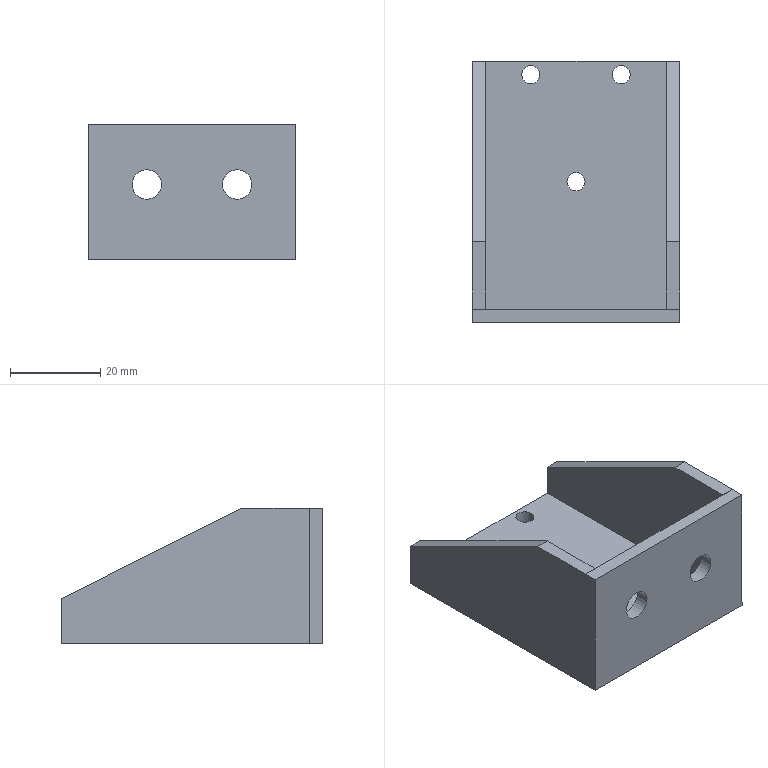Part | SolidWorks | features BaseBody 4 | 4 solids | 36 faces | box 46 x 58 x 30 mm | volume 17928 mm3 | plane 26 | cylinder 10 | commonest cylinder face diameters 4 x6 6.5 x4
STEP:
#1=CARTESIAN_POINT('',(-20.,-27.5,-1.5));
#2=VERTEX_POINT('',#1);
#3=CARTESIAN_POINT('',(-20.,27.5,-1.5));
#4=VERTEX_POINT('',#3);
#5=CARTESIAN_POINT('',(-20.,27.5,-1.5));
#6=DIRECTION('',(0.,1.,0.));
#7=VECTOR('',#6,1000.);
#8=LINE('',#5,#7);
#9=EDGE_CURVE('',#2,#4,#8,.T.);
#10=ORIENTED_EDGE('',*,*,#9,.T.);
#11=CARTESIAN_POINT('',(-20.,27.5,8.5));
#12=VERTEX_POINT('',#11);
#13=CARTESIAN_POINT('',(-20.,27.5,8.5));
#14=DIRECTION('',(0.,0.,1.));
#15=VECTOR('',#14,1000.);
#16=LINE('',#13,#15);
#17=EDGE_CURVE('',#4,#12,#16,.T.);
#18=ORIENTED_EDGE('',*,*,#17,.T.);
#19=CARTESIAN_POINT('',(-20.,-12.5,28.5));
#20=VERTEX_POINT('',#19);
#21=CARTESIAN_POINT('',(-20.,-12.5,28.5));
#22=DIRECTION('',(0.,-0.8944,0.4472));
#23=VECTOR('',#22,1000.);
#24=LINE('',#21,#23);
#25=EDGE_CURVE('',#12,#20,#24,.T.);
#26=ORIENTED_EDGE('',*,*,#25,.T.);
#27=CARTESIAN_POINT('',(-20.,-27.5,28.5));
#28=VERTEX_POINT('',#27);
#29=CARTESIAN_POINT('',(-20.,-27.5,28.5));
#30=DIRECTION('',(0.,-1.,0.));
#31=VECTOR('',#30,1000.);
#32=LINE('',#29,#31);
#33=EDGE_CURVE('',#20,#28,#32,.T.);
#34=ORIENTED_EDGE('',*,*,#33,.T.);
#35=CARTESIAN_POINT('',(-20.,-27.5,-1.5));
#36=DIRECTION('',(0.,0.,-1.));
#37=VECTOR('',#36,1000.);
#38=LINE('',#35,#37);
#39=EDGE_CURVE('',#28,#2,#38,.T.);
#40=ORIENTED_EDGE('',*,*,#39,.T.);
#41=EDGE_LOOP('',(#10,#18,#26,#34,#40));
#42=FACE_OUTER_BOUND('',#41,.T.);
#43=CARTESIAN_POINT('',(-20.,0.,0.));
#44=DIRECTION('',(-1.,0.,0.));
#45=DIRECTION('',(0.,0.,1.));
#46=AXIS2_PLACEMENT_3D('',#43,#44,#45);
#47=PLANE('',#46);
#48=ADVANCED_FACE('',(#42),#47,.F.);
#49=CARTESIAN_POINT('',(-23.,-27.5,28.5));
#50=VERTEX_POINT('',#49);
#51=CARTESIAN_POINT('',(-23.,-27.5,28.5));
#52=DIRECTION('',(-1.,0.,0.));
#53=VECTOR('',#52,1000.);
#54=LINE('',#51,#53);
#55=EDGE_CURVE('',#28,#50,#54,.T.);
#56=ORIENTED_EDGE('',*,*,#55,.T.);
#57=CARTESIAN_POINT('',(-23.,-27.5,-1.5));
#58=VERTEX_POINT('',#57);
#59=CARTESIAN_POINT('',(-23.,-27.5,0.));
#60=DIRECTION('',(0.,0.,1.));
#61=VECTOR('',#60,1000.);
#62=LINE('',#59,#61);
#63=EDGE_CURVE('',#58,#50,#62,.T.);
#64=ORIENTED_EDGE('',*,*,#63,.F.);
#65=CARTESIAN_POINT('',(-23.,-27.5,-1.5));
#66=DIRECTION('',(1.,0.,0.));
#67=VECTOR('',#66,1000.);
#68=LINE('',#65,#67);
#69=EDGE_CURVE('',#58,#2,#68,.T.);
#70=ORIENTED_EDGE('',*,*,#69,.T.);
#71=ORIENTED_EDGE('',*,*,#39,.F.);
#72=EDGE_LOOP('',(#56,#64,#70,#71));
#73=FACE_OUTER_BOUND('',#72,.T.);
#74=CARTESIAN_POINT('',(-23.,-27.5,-1.5));
#75=DIRECTION('',(0.,1.,0.));
#76=DIRECTION('',(1.,0.,0.));
#77=AXIS2_PLACEMENT_3D('',#74,#75,#76);
#78=PLANE('',#77);
#79=ADVANCED_FACE('',(#73),#78,.F.);
#80=CARTESIAN_POINT('',(-23.,-12.5,28.5));
#81=VERTEX_POINT('',#80);
#82=CARTESIAN_POINT('',(-23.,-12.5,28.5));
#83=DIRECTION('',(-1.,0.,0.));
#84=VECTOR('',#83,1000.);
#85=LINE('',#82,#84);
#86=EDGE_CURVE('',#20,#81,#85,.T.);
#87=ORIENTED_EDGE('',*,*,#86,.T.);
#88=CARTESIAN_POINT('',(-23.,0.,28.5));
#89=DIRECTION('',(0.,1.,0.));
#90=VECTOR('',#89,1000.);
#91=LINE('',#88,#90);
#92=EDGE_CURVE('',#50,#81,#91,.T.);
#93=ORIENTED_EDGE('',*,*,#92,.F.);
#94=ORIENTED_EDGE('',*,*,#55,.F.);
#95=ORIENTED_EDGE('',*,*,#33,.F.);
#96=EDGE_LOOP('',(#87,#93,#94,#95));
#97=FACE_OUTER_BOUND('',#96,.T.);
#98=CARTESIAN_POINT('',(-23.,-27.5,28.5));
#99=DIRECTION('',(0.,0.,-1.));
#100=DIRECTION('',(-1.,0.,0.));
#101=AXIS2_PLACEMENT_3D('',#98,#99,#100);
#102=PLANE('',#101);
#103=ADVANCED_FACE('',(#97),#102,.F.);
#104=CARTESIAN_POINT('',(-23.,27.5,8.5));
#105=VERTEX_POINT('',#104);
#106=CARTESIAN_POINT('',(-23.,27.5,8.5));
#107=DIRECTION('',(-1.,0.,0.));
#108=VECTOR('',#107,1000.);
#109=LINE('',#106,#108);
#110=EDGE_CURVE('',#12,#105,#109,.T.);
#111=ORIENTED_EDGE('',*,*,#110,.T.);
#112=CARTESIAN_POINT('',(-23.,-12.5,28.5));
#113=DIRECTION('',(0.,0.8944,-0.4472));
#114=VECTOR('',#113,1000.);
#115=LINE('',#112,#114);
#116=EDGE_CURVE('',#81,#105,#115,.T.);
#117=ORIENTED_EDGE('',*,*,#116,.F.);
#118=ORIENTED_EDGE('',*,*,#86,.F.);
#119=ORIENTED_EDGE('',*,*,#25,.F.);
#120=EDGE_LOOP('',(#111,#117,#118,#119));
#121=FACE_OUTER_BOUND('',#120,.T.);
#122=CARTESIAN_POINT('',(-23.,-12.5,28.5));
#123=DIRECTION('',(0.,-0.4472,-0.8944));
#124=DIRECTION('',(0.,-0.8944,0.4472));
#125=AXIS2_PLACEMENT_3D('',#122,#123,#124);
#126=PLANE('',#125);
#127=ADVANCED_FACE('',(#121),#126,.F.);
#128=CARTESIAN_POINT('',(-23.,27.5,-1.5));
#129=VERTEX_POINT('',#128);
#130=CARTESIAN_POINT('',(-23.,27.5,-1.5));
#131=DIRECTION('',(-1.,0.,0.));
#132=VECTOR('',#131,1000.);
#133=LINE('',#130,#132);
#134=EDGE_CURVE('',#4,#129,#133,.T.);
#135=ORIENTED_EDGE('',*,*,#134,.T.);
#136=CARTESIAN_POINT('',(-23.,27.5,0.));
#137=DIRECTION('',(0.,0.,-1.));
#138=VECTOR('',#137,1000.);
#139=LINE('',#136,#138);
#140=EDGE_CURVE('',#105,#129,#139,.T.);
#141=ORIENTED_EDGE('',*,*,#140,.F.);
#142=ORIENTED_EDGE('',*,*,#110,.F.);
#143=ORIENTED_EDGE('',*,*,#17,.F.);
#144=EDGE_LOOP('',(#135,#141,#142,#143));
#145=FACE_OUTER_BOUND('',#144,.T.);
#146=CARTESIAN_POINT('',(-23.,27.5,8.5));
#147=DIRECTION('',(0.,-1.,0.));
#148=DIRECTION('',(-1.,0.,0.));
#149=AXIS2_PLACEMENT_3D('',#146,#147,#148);
#150=PLANE('',#149);
#151=ADVANCED_FACE('',(#145),#150,.F.);
#152=ORIENTED_EDGE('',*,*,#69,.F.);
#153=CARTESIAN_POINT('',(-23.,0.,-1.5));
#154=DIRECTION('',(0.,-1.,0.));
#155=VECTOR('',#154,1000.);
#156=LINE('',#153,#155);
#157=EDGE_CURVE('',#129,#58,#156,.T.);
#158=ORIENTED_EDGE('',*,*,#157,.F.);
#159=ORIENTED_EDGE('',*,*,#134,.F.);
#160=ORIENTED_EDGE('',*,*,#9,.F.);
#161=EDGE_LOOP('',(#152,#158,#159,#160));
#162=FACE_OUTER_BOUND('',#161,.T.);
#163=CARTESIAN_POINT('',(-23.,27.5,-1.5));
#164=DIRECTION('',(0.,0.,1.));
#165=DIRECTION('',(1.,0.,0.));
#166=AXIS2_PLACEMENT_3D('',#163,#164,#165);
#167=PLANE('',#166);
#168=ADVANCED_FACE('',(#162),#167,.F.);
#169=ORIENTED_EDGE('',*,*,#140,.T.);
#170=ORIENTED_EDGE('',*,*,#157,.T.);
#171=ORIENTED_EDGE('',*,*,#63,.T.);
#172=ORIENTED_EDGE('',*,*,#92,.T.);
#173=ORIENTED_EDGE('',*,*,#116,.T.);
#174=EDGE_LOOP('',(#169,#170,#171,#172,#173));
#175=FACE_OUTER_BOUND('',#174,.T.);
#176=CARTESIAN_POINT('',(-23.,0.,0.));
#177=DIRECTION('',(-1.,0.,0.));
#178=DIRECTION('',(0.,0.,1.));
#179=AXIS2_PLACEMENT_3D('',#176,#177,#178);
#180=PLANE('',#179);
#181=ADVANCED_FACE('',(#175),#180,.T.);
#182=CLOSED_SHELL('',(#48,#79,#103,#127,#151,#168,#181));
#183=MANIFOLD_SOLID_BREP('',#182);
#184=CARTESIAN_POINT('',(6.75,-27.5,15.173));
#185=VERTEX_POINT('',#184);
#186=CARTESIAN_POINT('',(13.25,-27.5,15.173));
#187=VERTEX_POINT('',#186);
#188=CARTESIAN_POINT('',(10.,-27.5,15.173));
#189=DIRECTION('',(0.,-1.,0.));
#190=DIRECTION('',(-1.,0.,0.));
#191=AXIS2_PLACEMENT_3D('',#188,#189,#190);
#192=CIRCLE('',#191,3.25);
#193=EDGE_CURVE('',#185,#187,#192,.T.);
#194=ORIENTED_EDGE('',*,*,#193,.T.);
#195=CARTESIAN_POINT('',(10.,-27.5,15.173));
#196=DIRECTION('',(0.,-1.,0.));
#197=DIRECTION('',(-1.,0.,0.));
#198=AXIS2_PLACEMENT_3D('',#195,#196,#197);
#199=CIRCLE('',#198,3.25);
#200=EDGE_CURVE('',#187,#185,#199,.T.);
#201=ORIENTED_EDGE('',*,*,#200,.T.);
#202=EDGE_LOOP('',(#194,#201));
#203=FACE_BOUND('',#202,.T.);
#204=CARTESIAN_POINT('',(-13.25,-27.5,15.173));
#205=VERTEX_POINT('',#204);
#206=CARTESIAN_POINT('',(-6.75,-27.5,15.173));
#207=VERTEX_POINT('',#206);
#208=CARTESIAN_POINT('',(-10.,-27.5,15.173));
#209=DIRECTION('',(0.,-1.,0.));
#210=DIRECTION('',(-1.,0.,0.));
#211=AXIS2_PLACEMENT_3D('',#208,#209,#210);
#212=CIRCLE('',#211,3.25);
#213=EDGE_CURVE('',#205,#207,#212,.T.);
#214=ORIENTED_EDGE('',*,*,#213,.T.);
#215=CARTESIAN_POINT('',(-10.,-27.5,15.173));
#216=DIRECTION('',(0.,-1.,0.));
#217=DIRECTION('',(-1.,0.,0.));
#218=AXIS2_PLACEMENT_3D('',#215,#216,#217);
#219=CIRCLE('',#218,3.25);
#220=EDGE_CURVE('',#207,#205,#219,.T.);
#221=ORIENTED_EDGE('',*,*,#220,.T.);
#222=EDGE_LOOP('',(#214,#221));
#223=FACE_BOUND('',#222,.T.);
#224=CARTESIAN_POINT('',(23.,-27.5,28.5));
#225=VERTEX_POINT('',#224);
#226=CARTESIAN_POINT('',(23.,-27.5,-1.5));
#227=VERTEX_POINT('',#226);
#228=CARTESIAN_POINT('',(23.,-27.5,-1.5));
#229=DIRECTION('',(0.,0.,-1.));
#230=VECTOR('',#229,1000.);
#231=LINE('',#228,#230);
#232=EDGE_CURVE('',#225,#227,#231,.T.);
#233=ORIENTED_EDGE('',*,*,#232,.T.);
#234=CARTESIAN_POINT('',(-23.,-27.5,-1.5));
#235=VERTEX_POINT('',#234);
#236=CARTESIAN_POINT('',(-23.,-27.5,-1.5));
#237=DIRECTION('',(-1.,0.,0.));
#238=VECTOR('',#237,1000.);
#239=LINE('',#236,#238);
#240=EDGE_CURVE('',#227,#235,#239,.T.);
#241=ORIENTED_EDGE('',*,*,#240,.T.);
#242=CARTESIAN_POINT('',(-23.,-27.5,28.5));
#243=VERTEX_POINT('',#242);
#244=CARTESIAN_POINT('',(-23.,-27.5,-1.5));
#245=DIRECTION('',(0.,0.,1.));
#246=VECTOR('',#245,1000.);
#247=LINE('',#244,#246);
#248=EDGE_CURVE('',#235,#243,#247,.T.);
#249=ORIENTED_EDGE('',*,*,#248,.T.);
#250=CARTESIAN_POINT('',(-23.,-27.5,28.5));
#251=DIRECTION('',(1.,0.,0.));
#252=VECTOR('',#251,1000.);
#253=LINE('',#250,#252);
#254=EDGE_CURVE('',#243,#225,#253,.T.);
#255=ORIENTED_EDGE('',*,*,#254,.T.);
#256=EDGE_LOOP('',(#233,#241,#249,#255));
#257=FACE_OUTER_BOUND('',#256,.T.);
#258=CARTESIAN_POINT('',(0.,-27.5,0.));
#259=DIRECTION('',(0.,1.,0.));
#260=DIRECTION('',(1.,0.,0.));
#261=AXIS2_PLACEMENT_3D('',#258,#259,#260);
#262=PLANE('',#261);
#263=ADVANCED_FACE('',(#203,#223,#257),#262,.T.);
#264=CARTESIAN_POINT('',(13.25,-30.5,15.173));
#265=VERTEX_POINT('',#264);
#266=CARTESIAN_POINT('',(13.25,-40.5,15.173));
#267=DIRECTION('',(0.,1.,0.));
#268=VECTOR('',#267,1000.);
#269=LINE('',#266,#268);
#270=EDGE_CURVE('',#265,#187,#269,.T.);
#271=ORIENTED_EDGE('',*,*,#270,.F.);
#272=CARTESIAN_POINT('',(6.75,-30.5,15.173));
#273=VERTEX_POINT('',#272);
#274=CARTESIAN_POINT('',(10.,-30.5,15.173));
#275=DIRECTION('',(0.,-1.,0.));
#276=DIRECTION('',(-1.,0.,0.));
#277=AXIS2_PLACEMENT_3D('',#274,#275,#276);
#278=CIRCLE('',#277,3.25);
#279=EDGE_CURVE('',#265,#273,#278,.T.);
#280=ORIENTED_EDGE('',*,*,#279,.T.);
#281=CARTESIAN_POINT('',(6.75,-40.5,15.173));
#282=DIRECTION('',(0.,1.,0.));
#283=VECTOR('',#282,1000.);
#284=LINE('',#281,#283);
#285=EDGE_CURVE('',#273,#185,#284,.T.);
#286=ORIENTED_EDGE('',*,*,#285,.T.);
#287=ORIENTED_EDGE('',*,*,#200,.F.);
#288=EDGE_LOOP('',(#271,#280,#286,#287));
#289=FACE_OUTER_BOUND('',#288,.T.);
#290=CARTESIAN_POINT('',(10.,-40.5,15.173));
#291=DIRECTION('',(0.,1.,0.));
#292=DIRECTION('',(-1.,0.,0.));
#293=AXIS2_PLACEMENT_3D('',#290,#291,#292);
#294=CYLINDRICAL_SURFACE('',#293,3.25);
#295=ADVANCED_FACE('',(#289),#294,.F.);
#296=CARTESIAN_POINT('',(-6.75,-30.5,15.173));
#297=VERTEX_POINT('',#296);
#298=CARTESIAN_POINT('',(-6.75,-40.5,15.173));
#299=DIRECTION('',(0.,1.,0.));
#300=VECTOR('',#299,1000.);
#301=LINE('',#298,#300);
#302=EDGE_CURVE('',#297,#207,#301,.T.);
#303=ORIENTED_EDGE('',*,*,#302,.F.);
#304=CARTESIAN_POINT('',(-13.25,-30.5,15.173));
#305=VERTEX_POINT('',#304);
#306=CARTESIAN_POINT('',(-10.,-30.5,15.173));
#307=DIRECTION('',(0.,-1.,0.));
#308=DIRECTION('',(-1.,0.,0.));
#309=AXIS2_PLACEMENT_3D('',#306,#307,#308);
#310=CIRCLE('',#309,3.25);
#311=EDGE_CURVE('',#297,#305,#310,.T.);
#312=ORIENTED_EDGE('',*,*,#311,.T.);
#313=CARTESIAN_POINT('',(-13.25,-40.5,15.173));
#314=DIRECTION('',(0.,1.,0.));
#315=VECTOR('',#314,1000.);
#316=LINE('',#313,#315);
#317=EDGE_CURVE('',#305,#205,#316,.T.);
#318=ORIENTED_EDGE('',*,*,#317,.T.);
#319=ORIENTED_EDGE('',*,*,#220,.F.);
#320=EDGE_LOOP('',(#303,#312,#318,#319));
#321=FACE_OUTER_BOUND('',#320,.T.);
#322=CARTESIAN_POINT('',(-10.,-40.5,15.173));
#323=DIRECTION('',(0.,1.,0.));
#324=DIRECTION('',(-1.,0.,0.));
#325=AXIS2_PLACEMENT_3D('',#322,#323,#324);
#326=CYLINDRICAL_SURFACE('',#325,3.25);
#327=ADVANCED_FACE('',(#321),#326,.F.);
#328=CARTESIAN_POINT('',(-23.,-30.5,28.5));
#329=VERTEX_POINT('',#328);
#330=CARTESIAN_POINT('',(-23.,-30.5,28.5));
#331=DIRECTION('',(0.,-1.,0.));
#332=VECTOR('',#331,1000.);
#333=LINE('',#330,#332);
#334=EDGE_CURVE('',#243,#329,#333,.T.);
#335=ORIENTED_EDGE('',*,*,#334,.T.);
#336=CARTESIAN_POINT('',(23.,-30.5,28.5));
#337=VERTEX_POINT('',#336);
#338=CARTESIAN_POINT('',(0.,-30.5,28.5));
#339=DIRECTION('',(1.,0.,0.));
#340=VECTOR('',#339,1000.);
#341=LINE('',#338,#340);
#342=EDGE_CURVE('',#329,#337,#341,.T.);
#343=ORIENTED_EDGE('',*,*,#342,.T.);
#344=CARTESIAN_POINT('',(23.,-30.5,28.5));
#345=DIRECTION('',(0.,1.,0.));
#346=VECTOR('',#345,1000.);
#347=LINE('',#344,#346);
#348=EDGE_CURVE('',#337,#225,#347,.T.);
#349=ORIENTED_EDGE('',*,*,#348,.T.);
#350=ORIENTED_EDGE('',*,*,#254,.F.);
#351=EDGE_LOOP('',(#335,#343,#349,#350));
#352=FACE_OUTER_BOUND('',#351,.T.);
#353=CARTESIAN_POINT('',(-23.,-30.5,28.5));
#354=DIRECTION('',(0.,0.,-1.));
#355=DIRECTION('',(0.,-1.,0.));
#356=AXIS2_PLACEMENT_3D('',#353,#354,#355);
#357=PLANE('',#356);
#358=ADVANCED_FACE('',(#352),#357,.F.);
#359=ORIENTED_EDGE('',*,*,#348,.F.);
#360=CARTESIAN_POINT('',(23.,-30.5,-1.5));
#361=VERTEX_POINT('',#360);
#362=CARTESIAN_POINT('',(23.,-30.5,0.));
#363=DIRECTION('',(0.,0.,-1.));
#364=VECTOR('',#363,1000.);
#365=LINE('',#362,#364);
#366=EDGE_CURVE('',#337,#361,#365,.T.);
#367=ORIENTED_EDGE('',*,*,#366,.T.);
#368=CARTESIAN_POINT('',(23.,-30.5,-1.5));
#369=DIRECTION('',(0.,1.,0.));
#370=VECTOR('',#369,1000.);
#371=LINE('',#368,#370);
#372=EDGE_CURVE('',#361,#227,#371,.T.);
#373=ORIENTED_EDGE('',*,*,#372,.T.);
#374=ORIENTED_EDGE('',*,*,#232,.F.);
#375=EDGE_LOOP('',(#359,#367,#373,#374));
#376=FACE_OUTER_BOUND('',#375,.T.);
#377=CARTESIAN_POINT('',(23.,-30.5,-1.5));
#378=DIRECTION('',(-1.,0.,0.));
#379=DIRECTION('',(0.,1.,0.));
#380=AXIS2_PLACEMENT_3D('',#377,#378,#379);
#381=PLANE('',#380);
#382=ADVANCED_FACE('',(#376),#381,.F.);
#383=ORIENTED_EDGE('',*,*,#372,.F.);
#384=CARTESIAN_POINT('',(-23.,-30.5,-1.5));
#385=VERTEX_POINT('',#384);
#386=CARTESIAN_POINT('',(0.,-30.5,-1.5));
#387=DIRECTION('',(-1.,0.,0.));
#388=VECTOR('',#387,1000.);
#389=LINE('',#386,#388);
#390=EDGE_CURVE('',#361,#385,#389,.T.);
#391=ORIENTED_EDGE('',*,*,#390,.T.);
#392=CARTESIAN_POINT('',(-23.,-30.5,-1.5));
#393=DIRECTION('',(0.,1.,0.));
#394=VECTOR('',#393,1000.);
#395=LINE('',#392,#394);
#396=EDGE_CURVE('',#385,#235,#395,.T.);
#397=ORIENTED_EDGE('',*,*,#396,.T.);
#398=ORIENTED_EDGE('',*,*,#240,.F.);
#399=EDGE_LOOP('',(#383,#391,#397,#398));
#400=FACE_OUTER_BOUND('',#399,.T.);
#401=CARTESIAN_POINT('',(-23.,-30.5,-1.5));
#402=DIRECTION('',(0.,0.,1.));
#403=DIRECTION('',(1.,0.,0.));
#404=AXIS2_PLACEMENT_3D('',#401,#402,#403);
#405=PLANE('',#404);
#406=ADVANCED_FACE('',(#400),#405,.F.);
#407=ORIENTED_EDGE('',*,*,#396,.F.);
#408=CARTESIAN_POINT('',(-23.,-30.5,0.));
#409=DIRECTION('',(0.,0.,1.));
#410=VECTOR('',#409,1000.);
#411=LINE('',#408,#410);
#412=EDGE_CURVE('',#385,#329,#411,.T.);
#413=ORIENTED_EDGE('',*,*,#412,.T.);
#414=ORIENTED_EDGE('',*,*,#334,.F.);
#415=ORIENTED_EDGE('',*,*,#248,.F.);
#416=EDGE_LOOP('',(#407,#413,#414,#415));
#417=FACE_OUTER_BOUND('',#416,.T.);
#418=CARTESIAN_POINT('',(-23.,-30.5,-1.5));
#419=DIRECTION('',(1.,0.,0.));
#420=DIRECTION('',(0.,1.,0.));
#421=AXIS2_PLACEMENT_3D('',#418,#419,#420);
#422=PLANE('',#421);
#423=ADVANCED_FACE('',(#417),#422,.F.);
#424=CARTESIAN_POINT('',(10.,-30.5,15.173));
#425=DIRECTION('',(0.,-1.,0.));
#426=DIRECTION('',(-1.,0.,0.));
#427=AXIS2_PLACEMENT_3D('',#424,#425,#426);
#428=CIRCLE('',#427,3.25);
#429=EDGE_CURVE('',#273,#265,#428,.T.);
#430=ORIENTED_EDGE('',*,*,#429,.F.);
#431=ORIENTED_EDGE('',*,*,#279,.F.);
#432=EDGE_LOOP('',(#430,#431));
#433=FACE_BOUND('',#432,.T.);
#434=CARTESIAN_POINT('',(-10.,-30.5,15.173));
#435=DIRECTION('',(0.,-1.,0.));
#436=DIRECTION('',(-1.,0.,0.));
#437=AXIS2_PLACEMENT_3D('',#434,#435,#436);
#438=CIRCLE('',#437,3.25);
#439=EDGE_CURVE('',#305,#297,#438,.T.);
#440=ORIENTED_EDGE('',*,*,#439,.F.);
#441=ORIENTED_EDGE('',*,*,#311,.F.);
#442=EDGE_LOOP('',(#440,#441));
#443=FACE_BOUND('',#442,.T.);
#444=ORIENTED_EDGE('',*,*,#390,.F.);
#445=ORIENTED_EDGE('',*,*,#366,.F.);
#446=ORIENTED_EDGE('',*,*,#342,.F.);
#447=ORIENTED_EDGE('',*,*,#412,.F.);
#448=EDGE_LOOP('',(#444,#445,#446,#447));
#449=FACE_OUTER_BOUND('',#448,.T.);
#450=CARTESIAN_POINT('',(0.,-30.5,0.));
#451=DIRECTION('',(0.,1.,0.));
#452=DIRECTION('',(1.,0.,0.));
#453=AXIS2_PLACEMENT_3D('',#450,#451,#452);
#454=PLANE('',#453);
#455=ADVANCED_FACE('',(#433,#443,#449),#454,.F.);
#456=ORIENTED_EDGE('',*,*,#429,.T.);
#457=ORIENTED_EDGE('',*,*,#270,.T.);
#458=ORIENTED_EDGE('',*,*,#193,.F.);
#459=ORIENTED_EDGE('',*,*,#285,.F.);
#460=EDGE_LOOP('',(#456,#457,#458,#459));
#461=FACE_OUTER_BOUND('',#460,.T.);
#462=CARTESIAN_POINT('',(10.,-40.5,15.173));
#463=DIRECTION('',(0.,1.,0.));
#464=DIRECTION('',(-1.,0.,0.));
#465=AXIS2_PLACEMENT_3D('',#462,#463,#464);
#466=CYLINDRICAL_SURFACE('',#465,3.25);
#467=ADVANCED_FACE('',(#461),#466,.F.);
#468=ORIENTED_EDGE('',*,*,#439,.T.);
#469=ORIENTED_EDGE('',*,*,#302,.T.);
#470=ORIENTED_EDGE('',*,*,#213,.F.);
#471=ORIENTED_EDGE('',*,*,#317,.F.);
#472=EDGE_LOOP('',(#468,#469,#470,#471));
#473=FACE_OUTER_BOUND('',#472,.T.);
#474=CARTESIAN_POINT('',(-10.,-40.5,15.173));
#475=DIRECTION('',(0.,1.,0.));
#476=DIRECTION('',(-1.,0.,0.));
#477=AXIS2_PLACEMENT_3D('',#474,#475,#476);
#478=CYLINDRICAL_SURFACE('',#477,3.25);
#479=ADVANCED_FACE('',(#473),#478,.F.);
#480=CLOSED_SHELL('',(#263,#295,#327,#358,#382,#406,#423,#455,#467,#479));
#481=MANIFOLD_SOLID_BREP('',#480);
#482=CARTESIAN_POINT('',(12.,24.5,-1.5));
#483=VERTEX_POINT('',#482);
#484=CARTESIAN_POINT('',(8.,24.5,-1.5));
#485=VERTEX_POINT('',#484);
#486=CARTESIAN_POINT('',(10.,24.5,-1.5));
#487=DIRECTION('',(0.,0.,1.));
#488=DIRECTION('',(1.,0.,0.));
#489=AXIS2_PLACEMENT_3D('',#486,#487,#488);
#490=CIRCLE('',#489,2.);
#491=EDGE_CURVE('',#483,#485,#490,.T.);
#492=ORIENTED_EDGE('',*,*,#491,.T.);
#493=CARTESIAN_POINT('',(10.,24.5,-1.5));
#494=DIRECTION('',(0.,0.,1.));
#495=DIRECTION('',(1.,0.,0.));
#496=AXIS2_PLACEMENT_3D('',#493,#494,#495);
#497=CIRCLE('',#496,2.);
#498=EDGE_CURVE('',#485,#483,#497,.T.);
#499=ORIENTED_EDGE('',*,*,#498,.T.);
#500=EDGE_LOOP('',(#492,#499));
#501=FACE_BOUND('',#500,.T.);
#502=CARTESIAN_POINT('',(2.,0.8,-1.5));
#503=VERTEX_POINT('',#502);
#504=CARTESIAN_POINT('',(-2.,0.8,-1.5));
#505=VERTEX_POINT('',#504);
#506=CARTESIAN_POINT('',(0.,0.8,-1.5));
#507=DIRECTION('',(0.,0.,1.));
#508=DIRECTION('',(1.,0.,0.));
#509=AXIS2_PLACEMENT_3D('',#506,#507,#508);
#510=CIRCLE('',#509,2.);
#511=EDGE_CURVE('',#503,#505,#510,.T.);
#512=ORIENTED_EDGE('',*,*,#511,.T.);
#513=CARTESIAN_POINT('',(0.,0.8,-1.5));
#514=DIRECTION('',(0.,0.,1.));
#515=DIRECTION('',(1.,0.,0.));
#516=AXIS2_PLACEMENT_3D('',#513,#514,#515);
#517=CIRCLE('',#516,2.);
#518=EDGE_CURVE('',#505,#503,#517,.T.);
#519=ORIENTED_EDGE('',*,*,#518,.T.);
#520=EDGE_LOOP('',(#512,#519));
#521=FACE_BOUND('',#520,.T.);
#522=CARTESIAN_POINT('',(-8.,24.5,-1.5));
#523=VERTEX_POINT('',#522);
#524=CARTESIAN_POINT('',(-12.,24.5,-1.5));
#525=VERTEX_POINT('',#524);
#526=CARTESIAN_POINT('',(-10.,24.5,-1.5));
#527=DIRECTION('',(0.,0.,1.));
#528=DIRECTION('',(1.,0.,0.));
#529=AXIS2_PLACEMENT_3D('',#526,#527,#528);
#530=CIRCLE('',#529,2.);
#531=EDGE_CURVE('',#523,#525,#530,.T.);
#532=ORIENTED_EDGE('',*,*,#531,.T.);
#533=CARTESIAN_POINT('',(-10.,24.5,-1.5));
#534=DIRECTION('',(0.,0.,1.));
#535=DIRECTION('',(1.,0.,0.));
#536=AXIS2_PLACEMENT_3D('',#533,#534,#535);
#537=CIRCLE('',#536,2.);
#538=EDGE_CURVE('',#525,#523,#537,.T.);
#539=ORIENTED_EDGE('',*,*,#538,.T.);
#540=EDGE_LOOP('',(#532,#539));
#541=FACE_BOUND('',#540,.T.);
#542=CARTESIAN_POINT('',(-20.,27.5,-1.5));
#543=VERTEX_POINT('',#542);
#544=CARTESIAN_POINT('',(20.,27.5,-1.5));
#545=VERTEX_POINT('',#544);
#546=CARTESIAN_POINT('',(20.,27.5,-1.5));
#547=DIRECTION('',(1.,0.,0.));
#548=VECTOR('',#547,1000.);
#549=LINE('',#546,#548);
#550=EDGE_CURVE('',#543,#545,#549,.T.);
#551=ORIENTED_EDGE('',*,*,#550,.T.);
#552=CARTESIAN_POINT('',(20.,-27.5,-1.5));
#553=VERTEX_POINT('',#552);
#554=CARTESIAN_POINT('',(20.,-27.5,-1.5));
#555=DIRECTION('',(0.,-1.,0.));
#556=VECTOR('',#555,1000.);
#557=LINE('',#554,#556);
#558=EDGE_CURVE('',#545,#553,#557,.T.);
#559=ORIENTED_EDGE('',*,*,#558,.T.);
#560=CARTESIAN_POINT('',(-20.,-27.5,-1.5));
#561=VERTEX_POINT('',#560);
#562=CARTESIAN_POINT('',(20.,-27.5,-1.5));
#563=DIRECTION('',(-1.,0.,0.));
#564=VECTOR('',#563,1000.);
#565=LINE('',#562,#564);
#566=EDGE_CURVE('',#553,#561,#565,.T.);
#567=ORIENTED_EDGE('',*,*,#566,.T.);
#568=CARTESIAN_POINT('',(-20.,-27.5,-1.5));
#569=DIRECTION('',(0.,1.,0.));
#570=VECTOR('',#569,1000.);
#571=LINE('',#568,#570);
#572=EDGE_CURVE('',#561,#543,#571,.T.);
#573=ORIENTED_EDGE('',*,*,#572,.T.);
#574=EDGE_LOOP('',(#551,#559,#567,#573));
#575=FACE_OUTER_BOUND('',#574,.T.);
#576=CARTESIAN_POINT('',(0.,0.,-1.5));
#577=DIRECTION('',(0.,0.,1.));
#578=DIRECTION('',(1.,0.,0.));
#579=AXIS2_PLACEMENT_3D('',#576,#577,#578);
#580=PLANE('',#579);
#581=ADVANCED_FACE('',(#501,#521,#541,#575),#580,.F.);
#582=CARTESIAN_POINT('',(8.,24.5,1.5));
#583=VERTEX_POINT('',#582);
#584=CARTESIAN_POINT('',(8.,24.5,-11.5));
#585=DIRECTION('',(0.,0.,1.));
#586=VECTOR('',#585,1000.);
#587=LINE('',#584,#586);
#588=EDGE_CURVE('',#485,#583,#587,.T.);
#589=ORIENTED_EDGE('',*,*,#588,.F.);
#590=ORIENTED_EDGE('',*,*,#491,.F.);
#591=CARTESIAN_POINT('',(12.,24.5,1.5));
#592=VERTEX_POINT('',#591);
#593=CARTESIAN_POINT('',(12.,24.5,-11.5));
#594=DIRECTION('',(0.,0.,1.));
#595=VECTOR('',#594,1000.);
#596=LINE('',#593,#595);
#597=EDGE_CURVE('',#483,#592,#596,.T.);
#598=ORIENTED_EDGE('',*,*,#597,.T.);
#599=CARTESIAN_POINT('',(10.,24.5,1.5));
#600=DIRECTION('',(0.,0.,-1.));
#601=DIRECTION('',(1.,0.,0.));
#602=AXIS2_PLACEMENT_3D('',#599,#600,#601);
#603=CIRCLE('',#602,2.);
#604=EDGE_CURVE('',#583,#592,#603,.T.);
#605=ORIENTED_EDGE('',*,*,#604,.F.);
#606=EDGE_LOOP('',(#589,#590,#598,#605));
#607=FACE_OUTER_BOUND('',#606,.T.);
#608=CARTESIAN_POINT('',(10.,24.5,-11.5));
#609=DIRECTION('',(0.,0.,1.));
#610=DIRECTION('',(1.,0.,0.));
#611=AXIS2_PLACEMENT_3D('',#608,#609,#610);
#612=CYLINDRICAL_SURFACE('',#611,2.);
#613=ADVANCED_FACE('',(#607),#612,.F.);
#614=CARTESIAN_POINT('',(-2.,0.8,1.5));
#615=VERTEX_POINT('',#614);
#616=CARTESIAN_POINT('',(-2.,0.8,-11.5));
#617=DIRECTION('',(0.,0.,1.));
#618=VECTOR('',#617,1000.);
#619=LINE('',#616,#618);
#620=EDGE_CURVE('',#505,#615,#619,.T.);
#621=ORIENTED_EDGE('',*,*,#620,.F.);
#622=ORIENTED_EDGE('',*,*,#511,.F.);
#623=CARTESIAN_POINT('',(2.,0.8,1.5));
#624=VERTEX_POINT('',#623);
#625=CARTESIAN_POINT('',(2.,0.8,-11.5));
#626=DIRECTION('',(0.,0.,1.));
#627=VECTOR('',#626,1000.);
#628=LINE('',#625,#627);
#629=EDGE_CURVE('',#503,#624,#628,.T.);
#630=ORIENTED_EDGE('',*,*,#629,.T.);
#631=CARTESIAN_POINT('',(0.,0.8,1.5));
#632=DIRECTION('',(0.,0.,-1.));
#633=DIRECTION('',(1.,0.,0.));
#634=AXIS2_PLACEMENT_3D('',#631,#632,#633);
#635=CIRCLE('',#634,2.);
#636=EDGE_CURVE('',#615,#624,#635,.T.);
#637=ORIENTED_EDGE('',*,*,#636,.F.);
#638=EDGE_LOOP('',(#621,#622,#630,#637));
#639=FACE_OUTER_BOUND('',#638,.T.);
#640=CARTESIAN_POINT('',(0.,0.8,-11.5));
#641=DIRECTION('',(0.,0.,1.));
#642=DIRECTION('',(1.,0.,0.));
#643=AXIS2_PLACEMENT_3D('',#640,#641,#642);
#644=CYLINDRICAL_SURFACE('',#643,2.);
#645=ADVANCED_FACE('',(#639),#644,.F.);
#646=CARTESIAN_POINT('',(-12.,24.5,1.5));
#647=VERTEX_POINT('',#646);
#648=CARTESIAN_POINT('',(-12.,24.5,-11.5));
#649=DIRECTION('',(0.,0.,1.));
#650=VECTOR('',#649,1000.);
#651=LINE('',#648,#650);
#652=EDGE_CURVE('',#525,#647,#651,.T.);
#653=ORIENTED_EDGE('',*,*,#652,.F.);
#654=ORIENTED_EDGE('',*,*,#531,.F.);
#655=CARTESIAN_POINT('',(-8.,24.5,1.5));
#656=VERTEX_POINT('',#655);
#657=CARTESIAN_POINT('',(-8.,24.5,-11.5));
#658=DIRECTION('',(0.,0.,1.));
#659=VECTOR('',#658,1000.);
#660=LINE('',#657,#659);
#661=EDGE_CURVE('',#523,#656,#660,.T.);
#662=ORIENTED_EDGE('',*,*,#661,.T.);
#663=CARTESIAN_POINT('',(-10.,24.5,1.5));
#664=DIRECTION('',(0.,0.,-1.));
#665=DIRECTION('',(1.,0.,0.));
#666=AXIS2_PLACEMENT_3D('',#663,#664,#665);
#667=CIRCLE('',#666,2.);
#668=EDGE_CURVE('',#647,#656,#667,.T.);
#669=ORIENTED_EDGE('',*,*,#668,.F.);
#670=EDGE_LOOP('',(#653,#654,#662,#669));
#671=FACE_OUTER_BOUND('',#670,.T.);
#672=CARTESIAN_POINT('',(-10.,24.5,-11.5));
#673=DIRECTION('',(0.,0.,1.));
#674=DIRECTION('',(1.,0.,0.));
#675=AXIS2_PLACEMENT_3D('',#672,#673,#674);
#676=CYLINDRICAL_SURFACE('',#675,2.);
#677=ADVANCED_FACE('',(#671),#676,.F.);
#678=CARTESIAN_POINT('',(-20.,-27.5,1.5));
#679=VERTEX_POINT('',#678);
#680=CARTESIAN_POINT('',(-20.,-27.5,1.5));
#681=DIRECTION('',(0.,0.,1.));
#682=VECTOR('',#681,1000.);
#683=LINE('',#680,#682);
#684=EDGE_CURVE('',#561,#679,#683,.T.);
#685=ORIENTED_EDGE('',*,*,#684,.T.);
#686=CARTESIAN_POINT('',(-20.,27.5,1.5));
#687=VERTEX_POINT('',#686);
#688=CARTESIAN_POINT('',(-20.,0.,1.5));
#689=DIRECTION('',(0.,-1.,0.));
#690=VECTOR('',#689,1000.);
#691=LINE('',#688,#690);
#692=EDGE_CURVE('',#687,#679,#691,.T.);
#693=ORIENTED_EDGE('',*,*,#692,.F.);
#694=CARTESIAN_POINT('',(-20.,27.5,1.5));
#695=DIRECTION('',(0.,0.,-1.));
#696=VECTOR('',#695,1000.);
#697=LINE('',#694,#696);
#698=EDGE_CURVE('',#687,#543,#697,.T.);
#699=ORIENTED_EDGE('',*,*,#698,.T.);
#700=ORIENTED_EDGE('',*,*,#572,.F.);
#701=EDGE_LOOP('',(#685,#693,#699,#700));
#702=FACE_OUTER_BOUND('',#701,.T.);
#703=CARTESIAN_POINT('',(-20.,-27.5,1.5));
#704=DIRECTION('',(1.,0.,0.));
#705=DIRECTION('',(0.,1.,0.));
#706=AXIS2_PLACEMENT_3D('',#703,#704,#705);
#707=PLANE('',#706);
#708=ADVANCED_FACE('',(#702),#707,.F.);
#709=CARTESIAN_POINT('',(20.,-27.5,1.5));
#710=VERTEX_POINT('',#709);
#711=CARTESIAN_POINT('',(20.,-27.5,1.5));
#712=DIRECTION('',(0.,0.,1.));
#713=VECTOR('',#712,1000.);
#714=LINE('',#711,#713);
#715=EDGE_CURVE('',#553,#710,#714,.T.);
#716=ORIENTED_EDGE('',*,*,#715,.T.);
#717=CARTESIAN_POINT('',(0.,-27.5,1.5));
#718=DIRECTION('',(1.,0.,0.));
#719=VECTOR('',#718,1000.);
#720=LINE('',#717,#719);
#721=EDGE_CURVE('',#679,#710,#720,.T.);
#722=ORIENTED_EDGE('',*,*,#721,.F.);
#723=ORIENTED_EDGE('',*,*,#684,.F.);
#724=ORIENTED_EDGE('',*,*,#566,.F.);
#725=EDGE_LOOP('',(#716,#722,#723,#724));
#726=FACE_OUTER_BOUND('',#725,.T.);
#727=CARTESIAN_POINT('',(20.,-27.5,1.5));
#728=DIRECTION('',(0.,1.,0.));
#729=DIRECTION('',(1.,0.,0.));
#730=AXIS2_PLACEMENT_3D('',#727,#728,#729);
#731=PLANE('',#730);
#732=ADVANCED_FACE('',(#726),#731,.F.);
#733=CARTESIAN_POINT('',(20.,27.5,1.5));
#734=VERTEX_POINT('',#733);
#735=CARTESIAN_POINT('',(20.,27.5,1.5));
#736=DIRECTION('',(0.,0.,1.));
#737=VECTOR('',#736,1000.);
#738=LINE('',#735,#737);
#739=EDGE_CURVE('',#545,#734,#738,.T.);
#740=ORIENTED_EDGE('',*,*,#739,.T.);
#741=CARTESIAN_POINT('',(20.,0.,1.5));
#742=DIRECTION('',(0.,1.,0.));
#743=VECTOR('',#742,1000.);
#744=LINE('',#741,#743);
#745=EDGE_CURVE('',#710,#734,#744,.T.);
#746=ORIENTED_EDGE('',*,*,#745,.F.);
#747=ORIENTED_EDGE('',*,*,#715,.F.);
#748=ORIENTED_EDGE('',*,*,#558,.F.);
#749=EDGE_LOOP('',(#740,#746,#747,#748));
#750=FACE_OUTER_BOUND('',#749,.T.);
#751=CARTESIAN_POINT('',(20.,-27.5,1.5));
#752=DIRECTION('',(-1.,0.,0.));
#753=DIRECTION('',(0.,0.,1.));
#754=AXIS2_PLACEMENT_3D('',#751,#752,#753);
#755=PLANE('',#754);
#756=ADVANCED_FACE('',(#750),#755,.F.);
#757=ORIENTED_EDGE('',*,*,#698,.F.);
#758=CARTESIAN_POINT('',(0.,27.5,1.5));
#759=DIRECTION('',(-1.,0.,0.));
#760=VECTOR('',#759,1000.);
#761=LINE('',#758,#760);
#762=EDGE_CURVE('',#734,#687,#761,.T.);
#763=ORIENTED_EDGE('',*,*,#762,.F.);
#764=ORIENTED_EDGE('',*,*,#739,.F.);
#765=ORIENTED_EDGE('',*,*,#550,.F.);
#766=EDGE_LOOP('',(#757,#763,#764,#765));
#767=FACE_OUTER_BOUND('',#766,.T.);
#768=CARTESIAN_POINT('',(20.,27.5,1.5));
#769=DIRECTION('',(0.,-1.,0.));
#770=DIRECTION('',(0.,0.,-1.));
#771=AXIS2_PLACEMENT_3D('',#768,#769,#770);
#772=PLANE('',#771);
#773=ADVANCED_FACE('',(#767),#772,.F.);
#774=CARTESIAN_POINT('',(10.,24.5,1.5));
#775=DIRECTION('',(0.,0.,-1.));
#776=DIRECTION('',(1.,0.,0.));
#777=AXIS2_PLACEMENT_3D('',#774,#775,#776);
#778=CIRCLE('',#777,2.);
#779=EDGE_CURVE('',#592,#583,#778,.T.);
#780=ORIENTED_EDGE('',*,*,#779,.T.);
#781=ORIENTED_EDGE('',*,*,#604,.T.);
#782=EDGE_LOOP('',(#780,#781));
#783=FACE_BOUND('',#782,.T.);
#784=CARTESIAN_POINT('',(0.,0.8,1.5));
#785=DIRECTION('',(0.,0.,-1.));
#786=DIRECTION('',(1.,0.,0.));
#787=AXIS2_PLACEMENT_3D('',#784,#785,#786);
#788=CIRCLE('',#787,2.);
#789=EDGE_CURVE('',#624,#615,#788,.T.);
#790=ORIENTED_EDGE('',*,*,#789,.T.);
#791=ORIENTED_EDGE('',*,*,#636,.T.);
#792=EDGE_LOOP('',(#790,#791));
#793=FACE_BOUND('',#792,.T.);
#794=CARTESIAN_POINT('',(-10.,24.5,1.5));
#795=DIRECTION('',(0.,0.,-1.));
#796=DIRECTION('',(1.,0.,0.));
#797=AXIS2_PLACEMENT_3D('',#794,#795,#796);
#798=CIRCLE('',#797,2.);
#799=EDGE_CURVE('',#656,#647,#798,.T.);
#800=ORIENTED_EDGE('',*,*,#799,.T.);
#801=ORIENTED_EDGE('',*,*,#668,.T.);
#802=EDGE_LOOP('',(#800,#801));
#803=FACE_BOUND('',#802,.T.);
#804=ORIENTED_EDGE('',*,*,#745,.T.);
#805=ORIENTED_EDGE('',*,*,#762,.T.);
#806=ORIENTED_EDGE('',*,*,#692,.T.);
#807=ORIENTED_EDGE('',*,*,#721,.T.);
#808=EDGE_LOOP('',(#804,#805,#806,#807));
#809=FACE_OUTER_BOUND('',#808,.T.);
#810=CARTESIAN_POINT('',(0.,0.,1.5));
#811=DIRECTION('',(0.,0.,1.));
#812=DIRECTION('',(1.,0.,0.));
#813=AXIS2_PLACEMENT_3D('',#810,#811,#812);
#814=PLANE('',#813);
#815=ADVANCED_FACE('',(#783,#793,#803,#809),#814,.T.);
#816=ORIENTED_EDGE('',*,*,#498,.F.);
#817=ORIENTED_EDGE('',*,*,#588,.T.);
#818=ORIENTED_EDGE('',*,*,#779,.F.);
#819=ORIENTED_EDGE('',*,*,#597,.F.);
#820=EDGE_LOOP('',(#816,#817,#818,#819));
#821=FACE_OUTER_BOUND('',#820,.T.);
#822=CARTESIAN_POINT('',(10.,24.5,-11.5));
#823=DIRECTION('',(0.,0.,1.));
#824=DIRECTION('',(1.,0.,0.));
#825=AXIS2_PLACEMENT_3D('',#822,#823,#824);
#826=CYLINDRICAL_SURFACE('',#825,2.);
#827=ADVANCED_FACE('',(#821),#826,.F.);
#828=ORIENTED_EDGE('',*,*,#518,.F.);
#829=ORIENTED_EDGE('',*,*,#620,.T.);
#830=ORIENTED_EDGE('',*,*,#789,.F.);
#831=ORIENTED_EDGE('',*,*,#629,.F.);
#832=EDGE_LOOP('',(#828,#829,#830,#831));
#833=FACE_OUTER_BOUND('',#832,.T.);
#834=CARTESIAN_POINT('',(0.,0.8,-11.5));
#835=DIRECTION('',(0.,0.,1.));
#836=DIRECTION('',(1.,0.,0.));
#837=AXIS2_PLACEMENT_3D('',#834,#835,#836);
#838=CYLINDRICAL_SURFACE('',#837,2.);
#839=ADVANCED_FACE('',(#833),#838,.F.);
#840=ORIENTED_EDGE('',*,*,#538,.F.);
#841=ORIENTED_EDGE('',*,*,#652,.T.);
#842=ORIENTED_EDGE('',*,*,#799,.F.);
#843=ORIENTED_EDGE('',*,*,#661,.F.);
#844=EDGE_LOOP('',(#840,#841,#842,#843));
#845=FACE_OUTER_BOUND('',#844,.T.);
#846=CARTESIAN_POINT('',(-10.,24.5,-11.5));
#847=DIRECTION('',(0.,0.,1.));
#848=DIRECTION('',(1.,0.,0.));
#849=AXIS2_PLACEMENT_3D('',#846,#847,#848);
#850=CYLINDRICAL_SURFACE('',#849,2.);
#851=ADVANCED_FACE('',(#845),#850,.F.);
#852=CLOSED_SHELL('',(#581,#613,#645,#677,#708,#732,#756,#773,#815,#827,#839,#851));
#853=MANIFOLD_SOLID_BREP('',#852);
#854=CARTESIAN_POINT('',(20.,-27.5,-1.5));
#855=VERTEX_POINT('',#854);
#856=CARTESIAN_POINT('',(20.,-27.5,28.5));
#857=VERTEX_POINT('',#856);
#858=CARTESIAN_POINT('',(20.,-27.5,28.5));
#859=DIRECTION('',(0.,0.,1.));
#860=VECTOR('',#859,1000.);
#861=LINE('',#858,#860);
#862=EDGE_CURVE('',#855,#857,#861,.T.);
#863=ORIENTED_EDGE('',*,*,#862,.T.);
#864=CARTESIAN_POINT('',(20.,-12.5,28.5));
#865=VERTEX_POINT('',#864);
#866=CARTESIAN_POINT('',(20.,-12.5,28.5));
#867=DIRECTION('',(0.,1.,0.));
#868=VECTOR('',#867,1000.);
#869=LINE('',#866,#868);
#870=EDGE_CURVE('',#857,#865,#869,.T.);
#871=ORIENTED_EDGE('',*,*,#870,.T.);
#872=CARTESIAN_POINT('',(20.,27.5,8.5));
#873=VERTEX_POINT('',#872);
#874=CARTESIAN_POINT('',(20.,27.5,8.5));
#875=DIRECTION('',(0.,0.8944,-0.4472));
#876=VECTOR('',#875,1000.);
#877=LINE('',#874,#876);
#878=EDGE_CURVE('',#865,#873,#877,.T.);
#879=ORIENTED_EDGE('',*,*,#878,.T.);
#880=CARTESIAN_POINT('',(20.,27.5,-1.5));
#881=VERTEX_POINT('',#880);
#882=CARTESIAN_POINT('',(20.,27.5,-1.5));
#883=DIRECTION('',(0.,0.,-1.));
#884=VECTOR('',#883,1000.);
#885=LINE('',#882,#884);
#886=EDGE_CURVE('',#873,#881,#885,.T.);
#887=ORIENTED_EDGE('',*,*,#886,.T.);
#888=CARTESIAN_POINT('',(20.,-27.5,-1.5));
#889=DIRECTION('',(0.,-1.,0.));
#890=VECTOR('',#889,1000.);
#891=LINE('',#888,#890);
#892=EDGE_CURVE('',#881,#855,#891,.T.);
#893=ORIENTED_EDGE('',*,*,#892,.T.);
#894=EDGE_LOOP('',(#863,#871,#879,#887,#893));
#895=FACE_OUTER_BOUND('',#894,.T.);
#896=CARTESIAN_POINT('',(20.,0.,0.));
#897=DIRECTION('',(1.,0.,0.));
#898=DIRECTION('',(0.,1.,0.));
#899=AXIS2_PLACEMENT_3D('',#896,#897,#898);
#900=PLANE('',#899);
#901=ADVANCED_FACE('',(#895),#900,.F.);
#902=CARTESIAN_POINT('',(23.,27.5,-1.5));
#903=VERTEX_POINT('',#902);
#904=CARTESIAN_POINT('',(23.,27.5,-1.5));
#905=DIRECTION('',(1.,0.,0.));
#906=VECTOR('',#905,1000.);
#907=LINE('',#904,#906);
#908=EDGE_CURVE('',#881,#903,#907,.T.);
#909=ORIENTED_EDGE('',*,*,#908,.T.);
#910=CARTESIAN_POINT('',(23.,-27.5,-1.5));
#911=VERTEX_POINT('',#910);
#912=CARTESIAN_POINT('',(23.,0.,-1.5));
#913=DIRECTION('',(0.,1.,0.));
#914=VECTOR('',#913,1000.);
#915=LINE('',#912,#914);
#916=EDGE_CURVE('',#911,#903,#915,.T.);
#917=ORIENTED_EDGE('',*,*,#916,.F.);
#918=CARTESIAN_POINT('',(23.,-27.5,-1.5));
#919=DIRECTION('',(-1.,0.,0.));
#920=VECTOR('',#919,1000.);
#921=LINE('',#918,#920);
#922=EDGE_CURVE('',#911,#855,#921,.T.);
#923=ORIENTED_EDGE('',*,*,#922,.T.);
#924=ORIENTED_EDGE('',*,*,#892,.F.);
#925=EDGE_LOOP('',(#909,#917,#923,#924));
#926=FACE_OUTER_BOUND('',#925,.T.);
#927=CARTESIAN_POINT('',(23.,-27.5,-1.5));
#928=DIRECTION('',(0.,0.,1.));
#929=DIRECTION('',(1.,0.,0.));
#930=AXIS2_PLACEMENT_3D('',#927,#928,#929);
#931=PLANE('',#930);
#932=ADVANCED_FACE('',(#926),#931,.F.);
#933=CARTESIAN_POINT('',(23.,27.5,8.5));
#934=VERTEX_POINT('',#933);
#935=CARTESIAN_POINT('',(23.,27.5,8.5));
#936=DIRECTION('',(1.,0.,0.));
#937=VECTOR('',#936,1000.);
#938=LINE('',#935,#937);
#939=EDGE_CURVE('',#873,#934,#938,.T.);
#940=ORIENTED_EDGE('',*,*,#939,.T.);
#941=CARTESIAN_POINT('',(23.,27.5,0.));
#942=DIRECTION('',(0.,0.,1.));
#943=VECTOR('',#942,1000.);
#944=LINE('',#941,#943);
#945=EDGE_CURVE('',#903,#934,#944,.T.);
#946=ORIENTED_EDGE('',*,*,#945,.F.);
#947=ORIENTED_EDGE('',*,*,#908,.F.);
#948=ORIENTED_EDGE('',*,*,#886,.F.);
#949=EDGE_LOOP('',(#940,#946,#947,#948));
#950=FACE_OUTER_BOUND('',#949,.T.);
#951=CARTESIAN_POINT('',(23.,27.5,-1.5));
#952=DIRECTION('',(0.,-1.,0.));
#953=DIRECTION('',(0.,0.,-1.));
#954=AXIS2_PLACEMENT_3D('',#951,#952,#953);
#955=PLANE('',#954);
#956=ADVANCED_FACE('',(#950),#955,.F.);
#957=CARTESIAN_POINT('',(23.,-12.5,28.5));
#958=VERTEX_POINT('',#957);
#959=CARTESIAN_POINT('',(23.,-12.5,28.5));
#960=DIRECTION('',(1.,0.,0.));
#961=VECTOR('',#960,1000.);
#962=LINE('',#959,#961);
#963=EDGE_CURVE('',#865,#958,#962,.T.);
#964=ORIENTED_EDGE('',*,*,#963,.T.);
#965=CARTESIAN_POINT('',(23.,27.5,8.5));
#966=DIRECTION('',(0.,-0.8944,0.4472));
#967=VECTOR('',#966,1000.);
#968=LINE('',#965,#967);
#969=EDGE_CURVE('',#934,#958,#968,.T.);
#970=ORIENTED_EDGE('',*,*,#969,.F.);
#971=ORIENTED_EDGE('',*,*,#939,.F.);
#972=ORIENTED_EDGE('',*,*,#878,.F.);
#973=EDGE_LOOP('',(#964,#970,#971,#972));
#974=FACE_OUTER_BOUND('',#973,.T.);
#975=CARTESIAN_POINT('',(23.,27.5,8.5));
#976=DIRECTION('',(0.,-0.4472,-0.8944));
#977=DIRECTION('',(0.,-0.8944,0.4472));
#978=AXIS2_PLACEMENT_3D('',#975,#976,#977);
#979=PLANE('',#978);
#980=ADVANCED_FACE('',(#974),#979,.F.);
#981=CARTESIAN_POINT('',(23.,-27.5,28.5));
#982=VERTEX_POINT('',#981);
#983=CARTESIAN_POINT('',(23.,-27.5,28.5));
#984=DIRECTION('',(1.,0.,0.));
#985=VECTOR('',#984,1000.);
#986=LINE('',#983,#985);
#987=EDGE_CURVE('',#857,#982,#986,.T.);
#988=ORIENTED_EDGE('',*,*,#987,.T.);
#989=CARTESIAN_POINT('',(23.,0.,28.5));
#990=DIRECTION('',(0.,-1.,0.));
#991=VECTOR('',#990,1000.);
#992=LINE('',#989,#991);
#993=EDGE_CURVE('',#958,#982,#992,.T.);
#994=ORIENTED_EDGE('',*,*,#993,.F.);
#995=ORIENTED_EDGE('',*,*,#963,.F.);
#996=ORIENTED_EDGE('',*,*,#870,.F.);
#997=EDGE_LOOP('',(#988,#994,#995,#996));
#998=FACE_OUTER_BOUND('',#997,.T.);
#999=CARTESIAN_POINT('',(23.,-12.5,28.5));
#1000=DIRECTION('',(0.,0.,-1.));
#1001=DIRECTION('',(-1.,0.,0.));
#1002=AXIS2_PLACEMENT_3D('',#999,#1000,#1001);
#1003=PLANE('',#1002);
#1004=ADVANCED_FACE('',(#998),#1003,.F.);
#1005=ORIENTED_EDGE('',*,*,#922,.F.);
#1006=CARTESIAN_POINT('',(23.,-27.5,0.));
#1007=DIRECTION('',(0.,0.,-1.));
#1008=VECTOR('',#1007,1000.);
#1009=LINE('',#1006,#1008);
#1010=EDGE_CURVE('',#982,#911,#1009,.T.);
#1011=ORIENTED_EDGE('',*,*,#1010,.F.);
#1012=ORIENTED_EDGE('',*,*,#987,.F.);
#1013=ORIENTED_EDGE('',*,*,#862,.F.);
#1014=EDGE_LOOP('',(#1005,#1011,#1012,#1013));
#1015=FACE_OUTER_BOUND('',#1014,.T.);
#1016=CARTESIAN_POINT('',(23.,-27.5,28.5));
#1017=DIRECTION('',(0.,1.,0.));
#1018=DIRECTION('',(1.,0.,0.));
#1019=AXIS2_PLACEMENT_3D('',#1016,#1017,#1018);
#1020=PLANE('',#1019);
#1021=ADVANCED_FACE('',(#1015),#1020,.F.);
#1022=ORIENTED_EDGE('',*,*,#993,.T.);
#1023=ORIENTED_EDGE('',*,*,#1010,.T.);
#1024=ORIENTED_EDGE('',*,*,#916,.T.);
#1025=ORIENTED_EDGE('',*,*,#945,.T.);
#1026=ORIENTED_EDGE('',*,*,#969,.T.);
#1027=EDGE_LOOP('',(#1022,#1023,#1024,#1025,#1026));
#1028=FACE_OUTER_BOUND('',#1027,.T.);
#1029=CARTESIAN_POINT('',(23.,0.,0.));
#1030=DIRECTION('',(1.,0.,0.));
#1031=DIRECTION('',(0.,1.,0.));
#1032=AXIS2_PLACEMENT_3D('',#1029,#1030,#1031);
#1033=PLANE('',#1032);
#1034=ADVANCED_FACE('',(#1028),#1033,.T.);
#1035=CLOSED_SHELL('',(#901,#932,#956,#980,#1004,#1021,#1034));
#1036=MANIFOLD_SOLID_BREP('',#1035);
#1037=CARTESIAN_POINT('',(0.,0.,0.));
#1038=DIRECTION('',(0.,0.,1.));
#1039=DIRECTION('',(1.,0.,0.));
#1040=AXIS2_PLACEMENT_3D('',#1037,#1038,#1039);
#1041=(LENGTH_UNIT()NAMED_UNIT(*)SI_UNIT(.MILLI.,.METRE.));
#1042=UNCERTAINTY_MEASURE_WITH_UNIT(LENGTH_MEASURE(0.00001),#1041,'','');
#1043=(NAMED_UNIT(*)PLANE_ANGLE_UNIT()SI_UNIT($,.RADIAN.));
#1044=(NAMED_UNIT(*)SI_UNIT($,.STERADIAN.)SOLID_ANGLE_UNIT());
#1045=(GEOMETRIC_REPRESENTATION_CONTEXT(3)GLOBAL_UNCERTAINTY_ASSIGNED_CONTEXT((#1042))GLOBAL_UNIT_ASSIGNED_CONTEXT((#1041,#1043,#1044))REPRESENTATION_CONTEXT('',''));
#1046=ADVANCED_BREP_SHAPE_REPRESENTATION('',(#183,#481,#853,#1036,#1040),#1045);